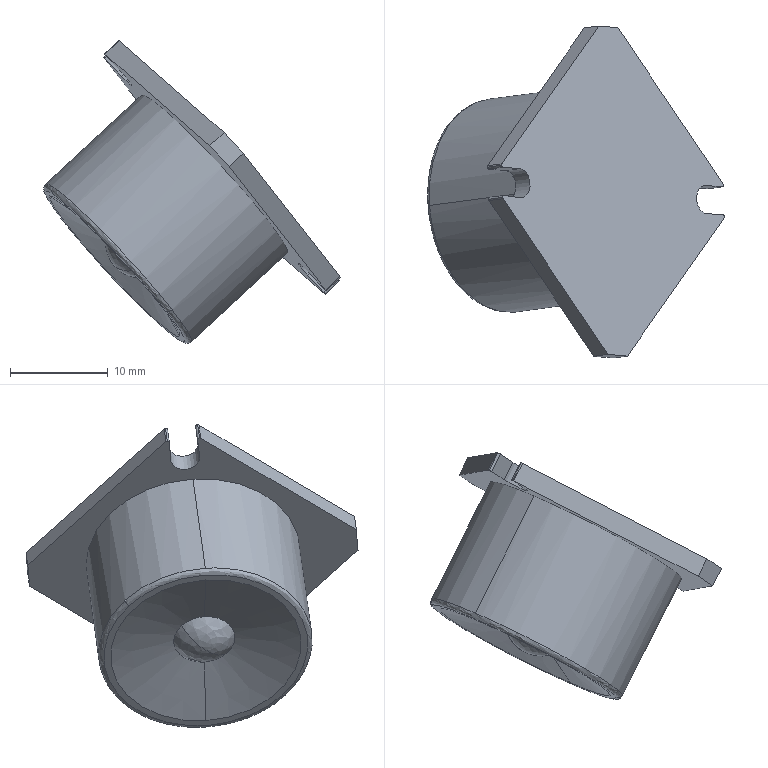Part | SolidWorks | features BaseBody 1 | 1 solid | 30 faces | box 30.403 x 34.026 x 31.023 mm | volume 6393 mm3 | plane 13 | cylinder 11 | spline 4 | cone 2 | commonest cylinder face diameters 0.4 x6 2.893 x2 22 x2 3.001 x1
STEP:
#1=CARTESIAN_POINT('',(690.687,-190.976,213.817));
#2=VERTEX_POINT('',#1);
#3=CARTESIAN_POINT('',(690.722,-190.926,213.773));
#4=VERTEX_POINT('',#3);
#5=CARTESIAN_POINT('',(690.687,-190.976,213.817));
#6=CARTESIAN_POINT('',(690.699,-190.959,213.802));
#7=CARTESIAN_POINT('',(690.71,-190.943,213.787));
#8=CARTESIAN_POINT('',(690.722,-190.926,213.773));
#9=(BOUNDED_CURVE()B_SPLINE_CURVE(3,(#5,#6,#7,#8),.UNSPECIFIED.,.F.,.F.)B_SPLINE_CURVE_WITH_KNOTS((4,4),(0.,0.002168),.UNSPECIFIED.)CURVE()GEOMETRIC_REPRESENTATION_ITEM()RATIONAL_B_SPLINE_CURVE((1.,1.,1.,1.))REPRESENTATION_ITEM(''));
#10=EDGE_CURVE('',#2,#4,#9,.T.);
#11=ORIENTED_EDGE('',*,*,#10,.T.);
#12=CARTESIAN_POINT('',(690.606,-191.348,213.217));
#13=VERTEX_POINT('',#12);
#14=CARTESIAN_POINT('',(690.722,-190.926,213.773));
#15=CARTESIAN_POINT('',(690.682,-190.932,213.735));
#16=CARTESIAN_POINT('',(690.597,-190.96,213.637));
#17=CARTESIAN_POINT('',(690.522,-191.062,213.467));
#18=CARTESIAN_POINT('',(690.529,-191.207,213.313));
#19=CARTESIAN_POINT('',(690.579,-191.307,213.241));
#20=CARTESIAN_POINT('',(690.606,-191.348,213.217));
#21=B_SPLINE_CURVE_WITH_KNOTS('',3,(#14,#15,#16,#17,#18,#19,#20),.UNSPECIFIED.,.F.,.F.,(4,1,1,1,4),(0.06704,0.25,0.5,0.75,0.933),.UNSPECIFIED.);
#22=EDGE_CURVE('',#4,#13,#21,.T.);
#23=ORIENTED_EDGE('',*,*,#22,.T.);
#24=CARTESIAN_POINT('',(690.573,-191.395,213.259));
#25=VERTEX_POINT('',#24);
#26=CARTESIAN_POINT('',(690.573,-191.395,213.259));
#27=CARTESIAN_POINT('',(690.584,-191.38,213.245));
#28=CARTESIAN_POINT('',(690.595,-191.364,213.231));
#29=CARTESIAN_POINT('',(690.606,-191.348,213.217));
#30=B_SPLINE_CURVE_WITH_KNOTS('',3,(#26,#27,#28,#29),.UNSPECIFIED.,.F.,.F.,(4,4),(0.,1.),.UNSPECIFIED.);
#31=EDGE_CURVE('',#25,#13,#30,.T.);
#32=ORIENTED_EDGE('',*,*,#31,.F.);
#33=CARTESIAN_POINT('',(701.095,-207.085,204.088));
#34=VERTEX_POINT('',#33);
#35=CARTESIAN_POINT('',(701.095,-207.085,204.088));
#36=CARTESIAN_POINT('',(700.775,-207.536,204.497));
#37=CARTESIAN_POINT('',(700.424,-207.933,204.932));
#38=CARTESIAN_POINT('',(699.662,-208.616,205.85));
#39=CARTESIAN_POINT('',(699.257,-208.897,206.327));
#40=CARTESIAN_POINT('',(698.403,-209.337,207.311));
#41=CARTESIAN_POINT('',(697.961,-209.491,207.811));
#42=CARTESIAN_POINT('',(697.047,-209.67,208.823));
#43=CARTESIAN_POINT('',(696.583,-209.692,209.327));
#44=CARTESIAN_POINT('',(695.645,-209.603,210.328));
#45=CARTESIAN_POINT('',(695.178,-209.492,210.817));
#46=CARTESIAN_POINT('',(694.251,-209.139,211.77));
#47=CARTESIAN_POINT('',(693.798,-208.899,212.225));
#48=CARTESIAN_POINT('',(692.918,-208.295,213.092));
#49=CARTESIAN_POINT('',(692.497,-207.936,213.496));
#50=CARTESIAN_POINT('',(691.697,-207.104,214.244));
#51=CARTESIAN_POINT('',(691.324,-206.638,214.582));
#52=CARTESIAN_POINT('',(690.635,-205.611,215.182));
#53=CARTESIAN_POINT('',(690.325,-205.057,215.44));
#54=CARTESIAN_POINT('',(689.773,-203.873,215.871));
#55=CARTESIAN_POINT('',(689.536,-203.253,216.039));
#56=CARTESIAN_POINT('',(689.143,-201.958,216.283));
#57=CARTESIAN_POINT('',(688.99,-201.294,216.356));
#58=CARTESIAN_POINT('',(688.77,-199.937,216.403));
#59=CARTESIAN_POINT('',(688.706,-199.255,216.377));
#60=CARTESIAN_POINT('',(688.668,-197.889,216.227));
#61=CARTESIAN_POINT('',(688.695,-197.215,216.103));
#62=CARTESIAN_POINT('',(688.841,-195.891,215.761));
#63=CARTESIAN_POINT('',(688.958,-195.252,215.544));
#64=CARTESIAN_POINT('',(689.282,-194.021,215.022));
#65=CARTESIAN_POINT('',(689.485,-193.44,214.721));
#66=CARTESIAN_POINT('',(689.974,-192.35,214.041));
#67=CARTESIAN_POINT('',(690.255,-191.85,213.667));
#68=CARTESIAN_POINT('',(690.573,-191.395,213.259));
#69=B_SPLINE_CURVE_WITH_KNOTS('',3,(#35,#36,#37,#38,#39,#40,#41,#42,#43,#44,#45,#46,#47,#48,#49,#50,#51,#52,#53,#54,#55,#56,#57,#58,#59,#60,#61,#62,#63,#64,#65,#66,#67,#68),.UNSPECIFIED.,.F.,.F.,(4,2,2,2,2,2,2,2,2,2,2,2,2,2,2,2,4),(0.,0.0625,0.125,0.1875,0.25,0.3125,0.375,0.4375,0.5,0.5625,0.625,0.6875,0.75,0.8125,0.875,0.9375,1.),.UNSPECIFIED.);
#70=EDGE_CURVE('',#34,#25,#69,.T.);
#71=ORIENTED_EDGE('',*,*,#70,.F.);
#72=CARTESIAN_POINT('',(701.71,-207.413,204.209));
#73=VERTEX_POINT('',#72);
#74=CARTESIAN_POINT('',(701.71,-207.413,204.209));
#75=CARTESIAN_POINT('',(701.669,-207.418,204.171));
#76=CARTESIAN_POINT('',(701.563,-207.414,204.092));
#77=CARTESIAN_POINT('',(701.376,-207.347,204.02));
#78=CARTESIAN_POINT('',(701.204,-207.223,204.022));
#79=CARTESIAN_POINT('',(701.123,-207.127,204.064));
#80=CARTESIAN_POINT('',(701.095,-207.085,204.088));
#81=B_SPLINE_CURVE_WITH_KNOTS('',3,(#74,#75,#76,#77,#78,#79,#80),.UNSPECIFIED.,.F.,.F.,(4,1,1,1,4),(0.06704,0.25,0.5,0.75,0.933),.UNSPECIFIED.);
#82=EDGE_CURVE('',#73,#34,#81,.T.);
#83=ORIENTED_EDGE('',*,*,#82,.F.);
#84=CARTESIAN_POINT('',(688.744,-199.17,217.063));
#85=VERTEX_POINT('',#84);
#86=CARTESIAN_POINT('',(701.71,-207.413,204.209));
#87=CARTESIAN_POINT('',(696.604,-214.6,210.731));
#88=CARTESIAN_POINT('',(689.506,-210.087,217.768));
#89=CARTESIAN_POINT('',(688.744,-199.17,217.063));
#90=(BOUNDED_CURVE()B_SPLINE_CURVE(3,(#86,#87,#88,#89),.UNSPECIFIED.,.F.,.F.)B_SPLINE_CURVE_WITH_KNOTS((4,4),(0.002168,0.7309),.UNSPECIFIED.)CURVE()GEOMETRIC_REPRESENTATION_ITEM()RATIONAL_B_SPLINE_CURVE((1.,0.6089,0.6089,1.))REPRESENTATION_ITEM(''));
#91=EDGE_CURVE('',#73,#85,#90,.T.);
#92=ORIENTED_EDGE('',*,*,#91,.T.);
#93=CARTESIAN_POINT('',(688.744,-199.17,217.063));
#94=CARTESIAN_POINT('',(688.522,-195.988,216.858));
#95=CARTESIAN_POINT('',(689.21,-193.086,215.708));
#96=CARTESIAN_POINT('',(690.687,-190.976,213.817));
#97=(BOUNDED_CURVE()B_SPLINE_CURVE(3,(#93,#94,#95,#96),.UNSPECIFIED.,.F.,.F.)B_SPLINE_CURVE_WITH_KNOTS((4,4),(0.7309,1.),.UNSPECIFIED.)CURVE()GEOMETRIC_REPRESENTATION_ITEM()RATIONAL_B_SPLINE_CURVE((1.,0.9413,0.9413,1.))REPRESENTATION_ITEM(''));
#98=EDGE_CURVE('',#85,#2,#97,.T.);
#99=ORIENTED_EDGE('',*,*,#98,.T.);
#100=EDGE_LOOP('',(#11,#23,#32,#71,#83,#92,#99));
#101=FACE_OUTER_BOUND('',#100,.T.);
#102=CARTESIAN_POINT('',(701.71,-207.413,204.209));
#103=CARTESIAN_POINT('',(691.467,-221.83,217.293));
#104=CARTESIAN_POINT('',(680.479,-205.344,226.857));
#105=CARTESIAN_POINT('',(690.722,-190.926,213.772));
#106=CARTESIAN_POINT('',(701.669,-207.418,204.171));
#107=CARTESIAN_POINT('',(691.426,-221.835,217.256));
#108=CARTESIAN_POINT('',(680.438,-205.349,226.82));
#109=CARTESIAN_POINT('',(690.682,-190.932,213.735));
#110=CARTESIAN_POINT('',(701.563,-207.414,204.092));
#111=CARTESIAN_POINT('',(691.34,-221.803,217.151));
#112=CARTESIAN_POINT('',(680.374,-205.349,226.696));
#113=CARTESIAN_POINT('',(690.597,-190.96,213.637));
#114=CARTESIAN_POINT('',(701.376,-207.347,204.02));
#115=CARTESIAN_POINT('',(691.257,-221.589,216.945));
#116=CARTESIAN_POINT('',(680.403,-205.303,226.392));
#117=CARTESIAN_POINT('',(690.522,-191.062,213.467));
#118=CARTESIAN_POINT('',(701.204,-207.223,204.022));
#119=CARTESIAN_POINT('',(691.253,-221.229,216.733));
#120=CARTESIAN_POINT('',(680.578,-205.213,226.024));
#121=CARTESIAN_POINT('',(690.529,-191.207,213.313));
#122=CARTESIAN_POINT('',(701.123,-207.127,204.064));
#123=CARTESIAN_POINT('',(691.293,-220.962,216.62));
#124=CARTESIAN_POINT('',(680.75,-205.142,225.797));
#125=CARTESIAN_POINT('',(690.579,-191.307,213.241));
#126=CARTESIAN_POINT('',(701.095,-207.085,204.088));
#127=CARTESIAN_POINT('',(691.317,-220.848,216.578));
#128=CARTESIAN_POINT('',(680.829,-205.111,225.707));
#129=CARTESIAN_POINT('',(690.606,-191.348,213.217));
#130=(BOUNDED_SURFACE()B_SPLINE_SURFACE(3,3,((#102,#103,#104,#105),(#106,#107,#108,#109),(#110,#111,#112,#113),(#114,#115,#116,#117),(#118,#119,#120,#121),(#122,#123,#124,#125),(#126,#127,#128,#129)),.UNSPECIFIED.,.F.,.F.,.T.)B_SPLINE_SURFACE_WITH_KNOTS((4,1,1,1,4),(4,4),(0.06704,0.25,0.5,0.75,0.933),(0.,1.),.UNSPECIFIED.)GEOMETRIC_REPRESENTATION_ITEM()RATIONAL_B_SPLINE_SURFACE(((1.,0.3333,0.3333,1.),(1.,0.3333,0.3333,1.),(1.,0.3333,0.3333,1.),(1.,0.3333,0.3333,1.),(1.,0.3333,0.3333,1.),(1.,0.3333,0.3333,1.),(1.,0.3333,0.3333,1.)))REPRESENTATION_ITEM('')SURFACE());
#131=ADVANCED_FACE('',(#101),#130,.F.);
#132=CARTESIAN_POINT('',(698.658,-201.411,208.396));
#133=VERTEX_POINT('',#132);
#134=CARTESIAN_POINT('',(699.215,-199.059,207.464));
#135=VERTEX_POINT('',#134);
#136=CARTESIAN_POINT('',(697.07,-199.059,209.781));
#137=DIRECTION('',(0.7306,0.09465,0.6762));
#138=DIRECTION('',(-0.5026,0.7449,0.4388));
#139=AXIS2_PLACEMENT_3D('',#136,#137,#138);
#140=CIRCLE('',#139,3.158);
#141=EDGE_CURVE('',#133,#135,#140,.T.);
#142=ORIENTED_EDGE('',*,*,#141,.F.);
#143=CARTESIAN_POINT('',(695.851,-199.217,208.652));
#144=VERTEX_POINT('',#143);
#145=CARTESIAN_POINT('',(698.658,-201.411,208.396));
#146=CARTESIAN_POINT('',(698.399,-201.312,208.305));
#147=CARTESIAN_POINT('',(697.861,-201.058,208.168));
#148=CARTESIAN_POINT('',(697.085,-200.545,208.134));
#149=CARTESIAN_POINT('',(696.385,-199.915,208.29));
#150=CARTESIAN_POINT('',(696.009,-199.452,208.514));
#151=CARTESIAN_POINT('',(695.851,-199.217,208.652));
#152=B_SPLINE_CURVE_WITH_KNOTS('',3,(#145,#146,#147,#148,#149,#150,#151),.UNSPECIFIED.,.F.,.F.,(4,1,1,1,4),(0.01961,0.25,0.5,0.75,1.),.UNSPECIFIED.);
#153=EDGE_CURVE('',#133,#144,#152,.T.);
#154=ORIENTED_EDGE('',*,*,#153,.T.);
#155=CARTESIAN_POINT('',(695.483,-196.707,211.167));
#156=VERTEX_POINT('',#155);
#157=CARTESIAN_POINT('',(695.483,-196.707,211.167));
#158=CARTESIAN_POINT('',(695.39,-196.851,210.932));
#159=CARTESIAN_POINT('',(695.253,-197.193,210.444));
#160=CARTESIAN_POINT('',(695.238,-197.808,209.747));
#161=CARTESIAN_POINT('',(695.432,-198.503,209.122));
#162=CARTESIAN_POINT('',(695.692,-198.982,208.791));
#163=CARTESIAN_POINT('',(695.851,-199.217,208.652));
#164=B_SPLINE_CURVE_WITH_KNOTS('',3,(#157,#158,#159,#160,#161,#162,#163),.UNSPECIFIED.,.F.,.F.,(4,1,1,1,4),(0.01961,0.25,0.5,0.75,1.),.UNSPECIFIED.);
#165=EDGE_CURVE('',#156,#144,#164,.T.);
#166=ORIENTED_EDGE('',*,*,#165,.F.);
#167=CARTESIAN_POINT('',(697.07,-199.059,209.781));
#168=DIRECTION('',(0.7306,0.09465,0.6762));
#169=DIRECTION('',(-0.5026,0.7449,0.4388));
#170=AXIS2_PLACEMENT_3D('',#167,#168,#169);
#171=CIRCLE('',#170,3.158);
#172=EDGE_CURVE('',#135,#156,#171,.T.);
#173=ORIENTED_EDGE('',*,*,#172,.F.);
#174=EDGE_LOOP('',(#142,#154,#166,#173));
#175=FACE_OUTER_BOUND('',#174,.T.);
#176=CARTESIAN_POINT('',(695.483,-196.707,211.167));
#177=CARTESIAN_POINT('',(698.402,-192.536,207.43));
#178=CARTESIAN_POINT('',(701.577,-197.24,204.658));
#179=CARTESIAN_POINT('',(698.658,-201.411,208.396));
#180=CARTESIAN_POINT('',(695.39,-196.851,210.932));
#181=CARTESIAN_POINT('',(698.157,-192.897,207.389));
#182=CARTESIAN_POINT('',(701.167,-197.357,204.762));
#183=CARTESIAN_POINT('',(698.399,-201.312,208.305));
#184=CARTESIAN_POINT('',(695.253,-197.193,210.444));
#185=CARTESIAN_POINT('',(697.651,-193.766,207.374));
#186=CARTESIAN_POINT('',(700.259,-197.631,205.097));
#187=CARTESIAN_POINT('',(697.861,-201.058,208.168));
#188=CARTESIAN_POINT('',(695.238,-197.808,209.747));
#189=CARTESIAN_POINT('',(696.937,-195.381,207.572));
#190=CARTESIAN_POINT('',(698.784,-198.118,205.959));
#191=CARTESIAN_POINT('',(697.085,-200.545,208.134));
#192=CARTESIAN_POINT('',(695.432,-198.503,209.122));
#193=CARTESIAN_POINT('',(696.308,-197.252,208.));
#194=CARTESIAN_POINT('',(697.261,-198.664,207.168));
#195=CARTESIAN_POINT('',(696.385,-199.915,208.29));
#196=CARTESIAN_POINT('',(695.692,-198.982,208.791));
#197=CARTESIAN_POINT('',(695.984,-198.564,208.417));
#198=CARTESIAN_POINT('',(696.301,-199.035,208.14));
#199=CARTESIAN_POINT('',(696.009,-199.452,208.514));
#200=CARTESIAN_POINT('',(695.851,-199.217,208.652));
#201=CARTESIAN_POINT('',(695.851,-199.217,208.652));
#202=CARTESIAN_POINT('',(695.851,-199.217,208.652));
#203=CARTESIAN_POINT('',(695.851,-199.217,208.652));
#204=(BOUNDED_SURFACE()B_SPLINE_SURFACE(3,3,((#176,#177,#178,#179),(#180,#181,#182,#183),(#184,#185,#186,#187),(#188,#189,#190,#191),(#192,#193,#194,#195),(#196,#197,#198,#199),(#200,#201,#202,#203)),.UNSPECIFIED.,.F.,.F.,.T.)B_SPLINE_SURFACE_WITH_KNOTS((4,1,1,1,4),(4,4),(0.01961,0.25,0.5,0.75,1.),(0.,1.),.UNSPECIFIED.)GEOMETRIC_REPRESENTATION_ITEM()RATIONAL_B_SPLINE_SURFACE(((1.,0.3333,0.3333,1.),(1.,0.3333,0.3333,1.),(1.,0.3333,0.3333,1.),(1.,0.3333,0.3333,1.),(1.,0.3333,0.3333,1.),(1.,0.3333,0.3333,1.),(1.,0.3333,0.3333,1.)))REPRESENTATION_ITEM('')SURFACE());
#205=ADVANCED_FACE('',(#175),#204,.F.);
#206=CARTESIAN_POINT('',(717.052,-197.111,209.113));
#207=VERTEX_POINT('',#206);
#208=CARTESIAN_POINT('',(716.114,-198.548,210.327));
#209=VERTEX_POINT('',#208);
#210=CARTESIAN_POINT('',(717.096,-198.548,209.266));
#211=DIRECTION('',(0.7306,0.09465,0.6762));
#212=DIRECTION('',(-0.6793,0.,0.7339));
#213=AXIS2_PLACEMENT_3D('',#210,#211,#212);
#214=CIRCLE('',#213,1.446);
#215=EDGE_CURVE('',#207,#209,#214,.T.);
#216=ORIENTED_EDGE('',*,*,#215,.T.);
#217=CARTESIAN_POINT('',(714.653,-198.738,208.975));
#218=VERTEX_POINT('',#217);
#219=CARTESIAN_POINT('',(716.114,-198.548,210.327));
#220=DIRECTION('',(-0.7306,-0.09465,-0.6762));
#221=VECTOR('',#220,1000.);
#222=LINE('',#219,#221);
#223=EDGE_CURVE('',#209,#218,#222,.T.);
#224=ORIENTED_EDGE('',*,*,#223,.T.);
#225=CARTESIAN_POINT('',(715.591,-197.3,207.76));
#226=VERTEX_POINT('',#225);
#227=CARTESIAN_POINT('',(715.635,-198.738,207.913));
#228=DIRECTION('',(-0.7306,-0.09465,-0.6762));
#229=DIRECTION('',(-0.6793,0.,0.7339));
#230=AXIS2_PLACEMENT_3D('',#227,#228,#229);
#231=CIRCLE('',#230,1.446);
#232=EDGE_CURVE('',#218,#226,#231,.T.);
#233=ORIENTED_EDGE('',*,*,#232,.T.);
#234=CARTESIAN_POINT('',(716.321,-197.205,208.437));
#235=DIRECTION('',(0.7306,0.09465,0.6762));
#236=VECTOR('',#235,1000.);
#237=LINE('',#234,#236);
#238=EDGE_CURVE('',#226,#207,#237,.T.);
#239=ORIENTED_EDGE('',*,*,#238,.T.);
#240=EDGE_LOOP('',(#216,#224,#233,#239));
#241=FACE_OUTER_BOUND('',#240,.T.);
#242=CARTESIAN_POINT('',(717.096,-198.548,209.266));
#243=DIRECTION('',(-0.7306,-0.09465,-0.6762));
#244=DIRECTION('',(-0.6793,0.,0.7339));
#245=AXIS2_PLACEMENT_3D('',#242,#243,#244);
#246=CYLINDRICAL_SURFACE('',#245,1.446);
#247=ADVANCED_FACE('',(#241),#246,.F.);
#248=CARTESIAN_POINT('',(696.132,-195.082,231.431));
#249=VERTEX_POINT('',#248);
#250=CARTESIAN_POINT('',(696.274,-195.281,231.305));
#251=VERTEX_POINT('',#250);
#252=CARTESIAN_POINT('',(696.268,-195.082,231.284));
#253=DIRECTION('',(0.7306,0.09465,0.6762));
#254=DIRECTION('',(-0.6793,0.,0.7339));
#255=AXIS2_PLACEMENT_3D('',#252,#253,#254);
#256=CIRCLE('',#255,0.2);
#257=EDGE_CURVE('',#249,#251,#256,.T.);
#258=ORIENTED_EDGE('',*,*,#257,.F.);
#259=CARTESIAN_POINT('',(694.671,-195.272,230.078));
#260=VERTEX_POINT('',#259);
#261=CARTESIAN_POINT('',(696.132,-195.082,231.431));
#262=DIRECTION('',(-0.7306,-0.09465,-0.6762));
#263=VECTOR('',#262,1000.);
#264=LINE('',#261,#263);
#265=EDGE_CURVE('',#249,#260,#264,.T.);
#266=ORIENTED_EDGE('',*,*,#265,.T.);
#267=CARTESIAN_POINT('',(694.813,-195.47,229.953));
#268=VERTEX_POINT('',#267);
#269=CARTESIAN_POINT('',(694.807,-195.272,229.931));
#270=DIRECTION('',(-0.7306,-0.09465,-0.6762));
#271=DIRECTION('',(-0.6793,0.,0.7339));
#272=AXIS2_PLACEMENT_3D('',#269,#270,#271);
#273=CIRCLE('',#272,0.2);
#274=EDGE_CURVE('',#268,#260,#273,.T.);
#275=ORIENTED_EDGE('',*,*,#274,.F.);
#276=CARTESIAN_POINT('',(695.543,-195.376,230.629));
#277=DIRECTION('',(0.7306,0.09465,0.6762));
#278=VECTOR('',#277,1000.);
#279=LINE('',#276,#278);
#280=EDGE_CURVE('',#268,#251,#279,.T.);
#281=ORIENTED_EDGE('',*,*,#280,.T.);
#282=EDGE_LOOP('',(#258,#266,#275,#281));
#283=FACE_OUTER_BOUND('',#282,.T.);
#284=CARTESIAN_POINT('',(696.268,-195.082,231.284));
#285=DIRECTION('',(-0.7306,-0.09465,-0.6762));
#286=DIRECTION('',(-0.6793,0.,0.7339));
#287=AXIS2_PLACEMENT_3D('',#284,#285,#286);
#288=CYLINDRICAL_SURFACE('',#287,0.2);
#289=ADVANCED_FACE('',(#283),#288,.T.);
#290=CARTESIAN_POINT('',(696.237,-198.374,231.778));
#291=VERTEX_POINT('',#290);
#292=CARTESIAN_POINT('',(696.28,-198.506,231.749));
#293=VERTEX_POINT('',#292);
#294=CARTESIAN_POINT('',(696.373,-198.374,231.631));
#295=DIRECTION('',(0.7306,0.09465,0.6762));
#296=DIRECTION('',(-0.6793,0.,0.7339));
#297=AXIS2_PLACEMENT_3D('',#294,#295,#296);
#298=CIRCLE('',#297,0.2);
#299=EDGE_CURVE('',#291,#293,#298,.T.);
#300=ORIENTED_EDGE('',*,*,#299,.F.);
#301=CARTESIAN_POINT('',(694.776,-198.563,230.425));
#302=VERTEX_POINT('',#301);
#303=CARTESIAN_POINT('',(696.237,-198.374,231.778));
#304=DIRECTION('',(-0.7306,-0.09465,-0.6762));
#305=VECTOR('',#304,1000.);
#306=LINE('',#303,#305);
#307=EDGE_CURVE('',#291,#302,#306,.T.);
#308=ORIENTED_EDGE('',*,*,#307,.T.);
#309=CARTESIAN_POINT('',(694.819,-198.695,230.397));
#310=VERTEX_POINT('',#309);
#311=CARTESIAN_POINT('',(694.912,-198.563,230.279));
#312=DIRECTION('',(-0.7306,-0.09465,-0.6762));
#313=DIRECTION('',(-0.6793,0.,0.7339));
#314=AXIS2_PLACEMENT_3D('',#311,#312,#313);
#315=CIRCLE('',#314,0.2);
#316=EDGE_CURVE('',#310,#302,#315,.T.);
#317=ORIENTED_EDGE('',*,*,#316,.F.);
#318=CARTESIAN_POINT('',(695.55,-198.6,231.073));
#319=DIRECTION('',(0.7306,0.09465,0.6762));
#320=VECTOR('',#319,1000.);
#321=LINE('',#318,#320);
#322=EDGE_CURVE('',#310,#293,#321,.T.);
#323=ORIENTED_EDGE('',*,*,#322,.T.);
#324=EDGE_LOOP('',(#300,#308,#317,#323));
#325=FACE_OUTER_BOUND('',#324,.T.);
#326=CARTESIAN_POINT('',(696.373,-198.374,231.631));
#327=DIRECTION('',(-0.7306,-0.09465,-0.6762));
#328=DIRECTION('',(-0.6793,0.,0.7339));
#329=AXIS2_PLACEMENT_3D('',#326,#327,#328);
#330=CYLINDRICAL_SURFACE('',#329,0.2);
#331=ADVANCED_FACE('',(#325),#330,.T.);
#332=CARTESIAN_POINT('',(713.551,-197.892,210.047));
#333=VERTEX_POINT('',#332);
#334=CARTESIAN_POINT('',(698.607,-197.892,226.192));
#335=VERTEX_POINT('',#334);
#336=CARTESIAN_POINT('',(706.079,-197.892,218.12));
#337=DIRECTION('',(0.7306,0.09465,0.6762));
#338=DIRECTION('',(-0.6793,0.,0.7339));
#339=AXIS2_PLACEMENT_3D('',#336,#337,#338);
#340=CIRCLE('',#339,11.);
#341=EDGE_CURVE('',#333,#335,#340,.T.);
#342=ORIENTED_EDGE('',*,*,#341,.F.);
#343=CARTESIAN_POINT('',(703.688,-199.17,200.918));
#344=VERTEX_POINT('',#343);
#345=CARTESIAN_POINT('',(713.551,-197.892,210.047));
#346=DIRECTION('',(-0.7306,-0.09465,-0.6762));
#347=VECTOR('',#346,1000.);
#348=LINE('',#345,#347);
#349=EDGE_CURVE('',#333,#344,#348,.T.);
#350=ORIENTED_EDGE('',*,*,#349,.T.);
#351=CARTESIAN_POINT('',(690.722,-190.926,213.773));
#352=CARTESIAN_POINT('',(695.828,-183.739,207.25));
#353=CARTESIAN_POINT('',(702.926,-188.252,200.213));
#354=CARTESIAN_POINT('',(703.688,-199.17,200.918));
#355=(BOUNDED_CURVE()B_SPLINE_CURVE(3,(#351,#352,#353,#354),.UNSPECIFIED.,.F.,.F.)B_SPLINE_CURVE_WITH_KNOTS((4,4),(0.002168,0.7309),.UNSPECIFIED.)CURVE()GEOMETRIC_REPRESENTATION_ITEM()RATIONAL_B_SPLINE_CURVE((1.,0.6089,0.6089,1.))REPRESENTATION_ITEM(''));
#356=EDGE_CURVE('',#4,#344,#355,.T.);
#357=ORIENTED_EDGE('',*,*,#356,.F.);
#358=ORIENTED_EDGE('',*,*,#10,.F.);
#359=ORIENTED_EDGE('',*,*,#98,.F.);
#360=CARTESIAN_POINT('',(698.607,-197.892,226.192));
#361=DIRECTION('',(-0.7306,-0.09465,-0.6762));
#362=VECTOR('',#361,1000.);
#363=LINE('',#360,#362);
#364=EDGE_CURVE('',#335,#85,#363,.T.);
#365=ORIENTED_EDGE('',*,*,#364,.F.);
#366=EDGE_LOOP('',(#342,#350,#357,#358,#359,#365));
#367=FACE_OUTER_BOUND('',#366,.T.);
#368=CARTESIAN_POINT('',(706.079,-197.892,218.12));
#369=DIRECTION('',(-0.7306,-0.09465,-0.6762));
#370=DIRECTION('',(-0.6793,0.,0.7339));
#371=AXIS2_PLACEMENT_3D('',#368,#369,#370);
#372=CYLINDRICAL_SURFACE('',#371,11.);
#373=ADVANCED_FACE('',(#367),#372,.T.);
#374=CARTESIAN_POINT('',(694.925,-199.059,212.099));
#375=VERTEX_POINT('',#374);
#376=CARTESIAN_POINT('',(697.07,-199.059,209.781));
#377=DIRECTION('',(0.7306,0.09465,0.6762));
#378=DIRECTION('',(-0.5026,0.7449,0.4388));
#379=AXIS2_PLACEMENT_3D('',#376,#377,#378);
#380=CIRCLE('',#379,3.158);
#381=EDGE_CURVE('',#375,#133,#380,.T.);
#382=ORIENTED_EDGE('',*,*,#381,.T.);
#383=ORIENTED_EDGE('',*,*,#141,.T.);
#384=CARTESIAN_POINT('',(702.52,-199.217,201.447));
#385=VERTEX_POINT('',#384);
#386=CARTESIAN_POINT('',(699.215,-199.059,207.464));
#387=DIRECTION('',(0.4812,-0.02301,-0.8763));
#388=VECTOR('',#387,1000.);
#389=LINE('',#386,#388);
#390=EDGE_CURVE('',#135,#385,#389,.T.);
#391=ORIENTED_EDGE('',*,*,#390,.T.);
#392=CARTESIAN_POINT('',(689.181,-199.217,215.858));
#393=VERTEX_POINT('',#392);
#394=CARTESIAN_POINT('',(695.851,-199.217,208.652));
#395=DIRECTION('',(0.7306,0.09465,0.6762));
#396=DIRECTION('',(-0.6793,0.,0.7339));
#397=AXIS2_PLACEMENT_3D('',#394,#395,#396);
#398=CIRCLE('',#397,9.818);
#399=EDGE_CURVE('',#393,#385,#398,.T.);
#400=ORIENTED_EDGE('',*,*,#399,.F.);
#401=CARTESIAN_POINT('',(694.925,-199.059,212.099));
#402=DIRECTION('',(-0.8365,-0.02301,0.5474));
#403=VECTOR('',#402,1000.);
#404=LINE('',#401,#403);
#405=EDGE_CURVE('',#375,#393,#404,.T.);
#406=ORIENTED_EDGE('',*,*,#405,.F.);
#407=EDGE_LOOP('',(#382,#383,#391,#400,#406));
#408=FACE_OUTER_BOUND('',#407,.T.);
#409=CARTESIAN_POINT('',(697.07,-199.059,209.781));
#410=DIRECTION('',(-0.7306,-0.09465,-0.6762));
#411=DIRECTION('',(-0.6793,0.,0.7339));
#412=AXIS2_PLACEMENT_3D('',#409,#410,#411);
#413=CONICAL_SURFACE('',#412,3.158,1.325);
#414=ADVANCED_FACE('',(#408),#413,.F.);
#415=CARTESIAN_POINT('',(697.969,-195.422,229.493));
#416=VERTEX_POINT('',#415);
#417=CARTESIAN_POINT('',(696.232,-195.278,231.349));
#418=DIRECTION('',(-0.6821,0.05658,0.729));
#419=VECTOR('',#418,1000.);
#420=LINE('',#417,#419);
#421=EDGE_CURVE('',#416,#251,#420,.T.);
#422=ORIENTED_EDGE('',*,*,#421,.F.);
#423=CARTESIAN_POINT('',(698.024,-198.4,229.851));
#424=VERTEX_POINT('',#423);
#425=CARTESIAN_POINT('',(698.016,-196.913,229.652));
#426=DIRECTION('',(0.7306,0.09465,0.6762));
#427=DIRECTION('',(-0.6793,0.,0.7339));
#428=AXIS2_PLACEMENT_3D('',#425,#426,#427);
#429=CIRCLE('',#428,1.501);
#430=EDGE_CURVE('',#424,#416,#429,.T.);
#431=ORIENTED_EDGE('',*,*,#430,.F.);
#432=CARTESIAN_POINT('',(696.372,-198.175,231.604));
#433=VERTEX_POINT('',#432);
#434=CARTESIAN_POINT('',(698.066,-198.406,229.807));
#435=DIRECTION('',(0.6828,-0.09294,-0.7247));
#436=VECTOR('',#435,1000.);
#437=LINE('',#434,#436);
#438=EDGE_CURVE('',#433,#424,#437,.T.);
#439=ORIENTED_EDGE('',*,*,#438,.F.);
#440=CARTESIAN_POINT('',(696.373,-198.374,231.631));
#441=DIRECTION('',(0.7306,0.09465,0.6762));
#442=DIRECTION('',(-0.6793,0.,0.7339));
#443=AXIS2_PLACEMENT_3D('',#440,#441,#442);
#444=CIRCLE('',#443,0.2);
#445=EDGE_CURVE('',#433,#291,#444,.T.);
#446=ORIENTED_EDGE('',*,*,#445,.T.);
#447=ORIENTED_EDGE('',*,*,#299,.T.);
#448=CARTESIAN_POINT('',(707.038,-214.448,222.359));
#449=VERTEX_POINT('',#448);
#450=CARTESIAN_POINT('',(701.532,-206.288,227.165));
#451=DIRECTION('',(-0.5026,0.7449,0.4388));
#452=VECTOR('',#451,1000.);
#453=LINE('',#450,#452);
#454=EDGE_CURVE('',#449,#293,#453,.T.);
#455=ORIENTED_EDGE('',*,*,#454,.F.);
#456=CARTESIAN_POINT('',(709.011,-214.621,220.251));
#457=VERTEX_POINT('',#456);
#458=CARTESIAN_POINT('',(706.996,-214.444,222.403));
#459=DIRECTION('',(-0.6822,0.05972,0.7287));
#460=VECTOR('',#459,1000.);
#461=LINE('',#458,#460);
#462=EDGE_CURVE('',#457,#449,#461,.T.);
#463=ORIENTED_EDGE('',*,*,#462,.F.);
#464=CARTESIAN_POINT('',(718.913,-200.472,207.572));
#465=VERTEX_POINT('',#464);
#466=CARTESIAN_POINT('',(714.074,-207.386,213.768));
#467=DIRECTION('',(-0.4622,-0.6604,0.5918));
#468=VECTOR('',#467,1000.);
#469=LINE('',#466,#468);
#470=EDGE_CURVE('',#465,#457,#469,.T.);
#471=ORIENTED_EDGE('',*,*,#470,.F.);
#472=CARTESIAN_POINT('',(718.806,-200.124,207.639));
#473=VERTEX_POINT('',#472);
#474=CARTESIAN_POINT('',(718.812,-200.323,207.66));
#475=DIRECTION('',(0.7306,0.09465,0.6762));
#476=DIRECTION('',(-0.6793,0.,0.7339));
#477=AXIS2_PLACEMENT_3D('',#474,#475,#476);
#478=CIRCLE('',#477,0.2);
#479=EDGE_CURVE('',#465,#473,#478,.T.);
#480=ORIENTED_EDGE('',*,*,#479,.T.);
#481=CARTESIAN_POINT('',(717.141,-199.986,209.419));
#482=VERTEX_POINT('',#481);
#483=CARTESIAN_POINT('',(718.848,-200.127,207.595));
#484=DIRECTION('',(0.6821,-0.05658,-0.729));
#485=VECTOR('',#484,1000.);
#486=LINE('',#483,#485);
#487=EDGE_CURVE('',#482,#473,#486,.T.);
#488=ORIENTED_EDGE('',*,*,#487,.F.);
#489=CARTESIAN_POINT('',(717.096,-198.548,209.266));
#490=DIRECTION('',(0.7306,0.09465,0.6762));
#491=DIRECTION('',(-0.6793,0.,0.7339));
#492=AXIS2_PLACEMENT_3D('',#489,#490,#491);
#493=CIRCLE('',#492,1.446);
#494=EDGE_CURVE('',#209,#482,#493,.T.);
#495=ORIENTED_EDGE('',*,*,#494,.F.);
#496=ORIENTED_EDGE('',*,*,#215,.F.);
#497=CARTESIAN_POINT('',(718.726,-197.25,207.323));
#498=VERTEX_POINT('',#497);
#499=CARTESIAN_POINT('',(717.01,-197.107,209.157));
#500=DIRECTION('',(-0.6821,0.05658,0.729));
#501=VECTOR('',#500,1000.);
#502=LINE('',#499,#501);
#503=EDGE_CURVE('',#498,#207,#502,.T.);
#504=ORIENTED_EDGE('',*,*,#503,.F.);
#505=CARTESIAN_POINT('',(718.813,-196.919,207.183));
#506=VERTEX_POINT('',#505);
#507=CARTESIAN_POINT('',(718.72,-197.051,207.302));
#508=DIRECTION('',(0.7306,0.09465,0.6762));
#509=DIRECTION('',(-0.6793,0.,0.7339));
#510=AXIS2_PLACEMENT_3D('',#507,#508,#509);
#511=CIRCLE('',#510,0.2);
#512=EDGE_CURVE('',#498,#506,#511,.T.);
#513=ORIENTED_EDGE('',*,*,#512,.T.);
#514=CARTESIAN_POINT('',(708.043,-180.957,216.585));
#515=VERTEX_POINT('',#514);
#516=CARTESIAN_POINT('',(713.549,-189.117,211.779));
#517=DIRECTION('',(0.5026,-0.7449,-0.4388));
#518=VECTOR('',#517,1000.);
#519=LINE('',#516,#518);
#520=EDGE_CURVE('',#515,#506,#519,.T.);
#521=ORIENTED_EDGE('',*,*,#520,.F.);
#522=CARTESIAN_POINT('',(706.069,-180.784,218.693));
#523=VERTEX_POINT('',#522);
#524=CARTESIAN_POINT('',(708.084,-180.961,216.541));
#525=DIRECTION('',(0.6822,-0.05972,-0.7287));
#526=VECTOR('',#525,1000.);
#527=LINE('',#524,#526);
#528=EDGE_CURVE('',#523,#515,#527,.T.);
#529=ORIENTED_EDGE('',*,*,#528,.F.);
#530=CARTESIAN_POINT('',(696.167,-194.933,231.372));
#531=VERTEX_POINT('',#530);
#532=CARTESIAN_POINT('',(701.006,-188.019,225.176));
#533=DIRECTION('',(0.4622,0.6604,-0.5918));
#534=VECTOR('',#533,1000.);
#535=LINE('',#532,#534);
#536=EDGE_CURVE('',#531,#523,#535,.T.);
#537=ORIENTED_EDGE('',*,*,#536,.F.);
#538=CARTESIAN_POINT('',(696.268,-195.082,231.284));
#539=DIRECTION('',(0.7306,0.09465,0.6762));
#540=DIRECTION('',(-0.6793,0.,0.7339));
#541=AXIS2_PLACEMENT_3D('',#538,#539,#540);
#542=CIRCLE('',#541,0.2);
#543=EDGE_CURVE('',#531,#249,#542,.T.);
#544=ORIENTED_EDGE('',*,*,#543,.T.);
#545=ORIENTED_EDGE('',*,*,#257,.T.);
#546=EDGE_LOOP('',(#422,#431,#439,#446,#447,#455,#463,#471,#480,#488,#495,#496,#504,#513,#521,#529,#537,#544,#545));
#547=FACE_OUTER_BOUND('',#546,.T.);
#548=CARTESIAN_POINT('',(708.087,-216.703,221.541));
#549=DIRECTION('',(-0.7306,-0.09465,-0.6762));
#550=DIRECTION('',(-0.5026,0.7449,0.4388));
#551=AXIS2_PLACEMENT_3D('',#548,#549,#550);
#552=PLANE('',#551);
#553=ADVANCED_FACE('',(#547),#552,.F.);
#554=CARTESIAN_POINT('',(696.508,-195.611,228.141));
#555=VERTEX_POINT('',#554);
#556=CARTESIAN_POINT('',(695.66,-195.541,229.047));
#557=DIRECTION('',(-0.6821,0.05658,0.729));
#558=VECTOR('',#557,1000.);
#559=LINE('',#556,#558);
#560=EDGE_CURVE('',#555,#268,#559,.T.);
#561=ORIENTED_EDGE('',*,*,#560,.F.);
#562=CARTESIAN_POINT('',(697.239,-195.516,228.817));
#563=DIRECTION('',(-0.7306,-0.09465,-0.6762));
#564=VECTOR('',#563,1000.);
#565=LINE('',#562,#564);
#566=EDGE_CURVE('',#416,#555,#565,.T.);
#567=ORIENTED_EDGE('',*,*,#566,.F.);
#568=ORIENTED_EDGE('',*,*,#421,.T.);
#569=ORIENTED_EDGE('',*,*,#280,.F.);
#570=EDGE_LOOP('',(#561,#567,#568,#569));
#571=FACE_OUTER_BOUND('',#570,.T.);
#572=CARTESIAN_POINT('',(696.277,-195.272,231.39));
#573=DIRECTION('',(-0.03074,0.9939,-0.1059));
#574=DIRECTION('',(0.6821,-0.05658,-0.729));
#575=AXIS2_PLACEMENT_3D('',#572,#573,#574);
#576=PLANE('',#575);
#577=ADVANCED_FACE('',(#571),#576,.F.);
#578=ORIENTED_EDGE('',*,*,#566,.T.);
#579=CARTESIAN_POINT('',(696.563,-198.59,228.498));
#580=VERTEX_POINT('',#579);
#581=CARTESIAN_POINT('',(696.554,-197.102,228.299));
#582=DIRECTION('',(-0.7306,-0.09465,-0.6762));
#583=DIRECTION('',(-0.6793,0.,0.7339));
#584=AXIS2_PLACEMENT_3D('',#581,#582,#583);
#585=CIRCLE('',#584,1.501);
#586=EDGE_CURVE('',#555,#580,#585,.T.);
#587=ORIENTED_EDGE('',*,*,#586,.T.);
#588=CARTESIAN_POINT('',(697.294,-198.495,229.175));
#589=DIRECTION('',(0.7306,0.09465,0.6762));
#590=VECTOR('',#589,1000.);
#591=LINE('',#588,#590);
#592=EDGE_CURVE('',#580,#424,#591,.T.);
#593=ORIENTED_EDGE('',*,*,#592,.T.);
#594=ORIENTED_EDGE('',*,*,#430,.T.);
#595=EDGE_LOOP('',(#578,#587,#593,#594));
#596=FACE_OUTER_BOUND('',#595,.T.);
#597=CARTESIAN_POINT('',(698.016,-196.913,229.652));
#598=DIRECTION('',(-0.7306,-0.09465,-0.6762));
#599=DIRECTION('',(-0.6793,0.,0.7339));
#600=AXIS2_PLACEMENT_3D('',#597,#598,#599);
#601=CYLINDRICAL_SURFACE('',#600,1.501);
#602=ADVANCED_FACE('',(#596),#601,.F.);
#603=ORIENTED_EDGE('',*,*,#438,.T.);
#604=ORIENTED_EDGE('',*,*,#592,.F.);
#605=CARTESIAN_POINT('',(694.911,-198.365,230.252));
#606=VERTEX_POINT('',#605);
#607=CARTESIAN_POINT('',(695.737,-198.477,229.375));
#608=DIRECTION('',(0.6828,-0.09294,-0.7247));
#609=VECTOR('',#608,1000.);
#610=LINE('',#607,#609);
#611=EDGE_CURVE('',#606,#580,#610,.T.);
#612=ORIENTED_EDGE('',*,*,#611,.F.);
#613=CARTESIAN_POINT('',(695.641,-198.27,230.928));
#614=DIRECTION('',(-0.7306,-0.09465,-0.6762));
#615=VECTOR('',#614,1000.);
#616=LINE('',#613,#615);
#617=EDGE_CURVE('',#433,#606,#616,.T.);
#618=ORIENTED_EDGE('',*,*,#617,.F.);
#619=EDGE_LOOP('',(#603,#604,#612,#618));
#620=FACE_OUTER_BOUND('',#619,.T.);
#621=CARTESIAN_POINT('',(698.11,-198.4,229.848));
#622=DIRECTION('',(0.005744,-0.9912,0.1325));
#623=DIRECTION('',(-0.6828,0.09294,0.7247));
#624=AXIS2_PLACEMENT_3D('',#621,#622,#623);
#625=PLANE('',#624);
#626=ADVANCED_FACE('',(#620),#625,.F.);
#627=CARTESIAN_POINT('',(705.576,-214.637,221.006));
#628=VERTEX_POINT('',#627);
#629=CARTESIAN_POINT('',(700.198,-206.666,225.702));
#630=DIRECTION('',(-0.5026,0.7449,0.4388));
#631=VECTOR('',#630,1000.);
#632=LINE('',#629,#631);
#633=EDGE_CURVE('',#628,#310,#632,.T.);
#634=ORIENTED_EDGE('',*,*,#633,.F.);
#635=CARTESIAN_POINT('',(706.307,-214.543,221.683));
#636=DIRECTION('',(-0.7306,-0.09465,-0.6762));
#637=VECTOR('',#636,1000.);
#638=LINE('',#635,#637);
#639=EDGE_CURVE('',#449,#628,#638,.T.);
#640=ORIENTED_EDGE('',*,*,#639,.F.);
#641=ORIENTED_EDGE('',*,*,#454,.T.);
#642=ORIENTED_EDGE('',*,*,#322,.F.);
#643=EDGE_LOOP('',(#634,#640,#641,#642));
#644=FACE_OUTER_BOUND('',#643,.T.);
#645=CARTESIAN_POINT('',(696.11,-198.181,231.978));
#646=DIRECTION('',(0.4622,0.6604,-0.5918));
#647=DIRECTION('',(0.5026,-0.7449,-0.4388));
#648=AXIS2_PLACEMENT_3D('',#645,#646,#647);
#649=PLANE('',#648);
#650=ADVANCED_FACE('',(#644),#649,.F.);
#651=CARTESIAN_POINT('',(707.55,-214.81,218.898));
#652=VERTEX_POINT('',#651);
#653=CARTESIAN_POINT('',(708.28,-214.715,219.575));
#654=DIRECTION('',(-0.7306,-0.09465,-0.6762));
#655=VECTOR('',#654,1000.);
#656=LINE('',#653,#655);
#657=EDGE_CURVE('',#457,#652,#656,.T.);
#658=ORIENTED_EDGE('',*,*,#657,.F.);
#659=ORIENTED_EDGE('',*,*,#462,.T.);
#660=ORIENTED_EDGE('',*,*,#639,.T.);
#661=CARTESIAN_POINT('',(706.563,-214.724,219.952));
#662=DIRECTION('',(-0.6822,0.05972,0.7287));
#663=VECTOR('',#662,1000.);
#664=LINE('',#661,#663);
#665=EDGE_CURVE('',#652,#628,#664,.T.);
#666=ORIENTED_EDGE('',*,*,#665,.F.);
#667=EDGE_LOOP('',(#658,#659,#660,#666));
#668=FACE_OUTER_BOUND('',#667,.T.);
#669=CARTESIAN_POINT('',(707.04,-214.439,222.444));
#670=DIRECTION('',(-0.02858,0.9937,-0.1082));
#671=DIRECTION('',(0.6822,-0.05972,-0.7287));
#672=AXIS2_PLACEMENT_3D('',#669,#670,#671);
#673=PLANE('',#672);
#674=ADVANCED_FACE('',(#668),#673,.F.);
#675=ORIENTED_EDGE('',*,*,#470,.T.);
#676=ORIENTED_EDGE('',*,*,#657,.T.);
#677=CARTESIAN_POINT('',(717.452,-200.661,206.22));
#678=VERTEX_POINT('',#677);
#679=CARTESIAN_POINT('',(712.501,-207.736,212.559));
#680=DIRECTION('',(-0.4622,-0.6604,0.5918));
#681=VECTOR('',#680,1000.);
#682=LINE('',#679,#681);
#683=EDGE_CURVE('',#678,#652,#682,.T.);
#684=ORIENTED_EDGE('',*,*,#683,.F.);
#685=CARTESIAN_POINT('',(718.182,-200.566,206.896));
#686=DIRECTION('',(-0.7306,-0.09465,-0.6762));
#687=VECTOR('',#686,1000.);
#688=LINE('',#685,#687);
#689=EDGE_CURVE('',#465,#678,#688,.T.);
#690=ORIENTED_EDGE('',*,*,#689,.F.);
#691=EDGE_LOOP('',(#675,#676,#684,#690));
#692=FACE_OUTER_BOUND('',#691,.T.);
#693=CARTESIAN_POINT('',(708.857,-214.898,220.546));
#694=DIRECTION('',(-0.5026,0.7449,0.4388));
#695=DIRECTION('',(0.4622,0.6604,-0.5918));
#696=AXIS2_PLACEMENT_3D('',#693,#694,#695);
#697=PLANE('',#696);
#698=ADVANCED_FACE('',(#692),#697,.F.);
#699=CARTESIAN_POINT('',(715.68,-200.175,208.067));
#700=VERTEX_POINT('',#699);
#701=CARTESIAN_POINT('',(717.345,-200.313,206.287));
#702=VERTEX_POINT('',#701);
#703=CARTESIAN_POINT('',(716.512,-200.244,207.177));
#704=DIRECTION('',(0.6821,-0.05658,-0.729));
#705=VECTOR('',#704,1000.);
#706=LINE('',#703,#705);
#707=EDGE_CURVE('',#700,#702,#706,.T.);
#708=ORIENTED_EDGE('',*,*,#707,.F.);
#709=CARTESIAN_POINT('',(716.41,-200.081,208.743));
#710=DIRECTION('',(-0.7306,-0.09465,-0.6762));
#711=VECTOR('',#710,1000.);
#712=LINE('',#709,#711);
#713=EDGE_CURVE('',#482,#700,#712,.T.);
#714=ORIENTED_EDGE('',*,*,#713,.F.);
#715=ORIENTED_EDGE('',*,*,#487,.T.);
#716=CARTESIAN_POINT('',(718.076,-200.219,206.963));
#717=DIRECTION('',(0.7306,0.09465,0.6762));
#718=VECTOR('',#717,1000.);
#719=LINE('',#716,#718);
#720=EDGE_CURVE('',#702,#473,#719,.T.);
#721=ORIENTED_EDGE('',*,*,#720,.F.);
#722=EDGE_LOOP('',(#708,#714,#715,#721));
#723=FACE_OUTER_BOUND('',#722,.T.);
#724=CARTESIAN_POINT('',(718.892,-200.122,207.636));
#725=DIRECTION('',(0.03074,-0.9939,0.1059));
#726=DIRECTION('',(-0.6821,0.05658,0.729));
#727=AXIS2_PLACEMENT_3D('',#724,#725,#726);
#728=PLANE('',#727);
#729=ADVANCED_FACE('',(#723),#728,.F.);
#730=ORIENTED_EDGE('',*,*,#223,.F.);
#731=ORIENTED_EDGE('',*,*,#494,.T.);
#732=ORIENTED_EDGE('',*,*,#713,.T.);
#733=CARTESIAN_POINT('',(715.635,-198.738,207.913));
#734=DIRECTION('',(-0.7306,-0.09465,-0.6762));
#735=DIRECTION('',(-0.6793,0.,0.7339));
#736=AXIS2_PLACEMENT_3D('',#733,#734,#735);
#737=CIRCLE('',#736,1.446);
#738=EDGE_CURVE('',#700,#218,#737,.T.);
#739=ORIENTED_EDGE('',*,*,#738,.T.);
#740=EDGE_LOOP('',(#730,#731,#732,#739));
#741=FACE_OUTER_BOUND('',#740,.T.);
#742=CARTESIAN_POINT('',(717.096,-198.548,209.266));
#743=DIRECTION('',(-0.7306,-0.09465,-0.6762));
#744=DIRECTION('',(-0.6793,0.,0.7339));
#745=AXIS2_PLACEMENT_3D('',#742,#743,#744);
#746=CYLINDRICAL_SURFACE('',#745,1.446);
#747=ADVANCED_FACE('',(#741),#746,.F.);
#748=ORIENTED_EDGE('',*,*,#503,.T.);
#749=ORIENTED_EDGE('',*,*,#238,.F.);
#750=CARTESIAN_POINT('',(717.265,-197.439,205.97));
#751=VERTEX_POINT('',#750);
#752=CARTESIAN_POINT('',(716.428,-197.369,206.865));
#753=DIRECTION('',(-0.6821,0.05658,0.729));
#754=VECTOR('',#753,1000.);
#755=LINE('',#752,#754);
#756=EDGE_CURVE('',#751,#226,#755,.T.);
#757=ORIENTED_EDGE('',*,*,#756,.F.);
#758=CARTESIAN_POINT('',(717.996,-197.344,206.647));
#759=DIRECTION('',(-0.7306,-0.09465,-0.6762));
#760=VECTOR('',#759,1000.);
#761=LINE('',#758,#760);
#762=EDGE_CURVE('',#498,#751,#761,.T.);
#763=ORIENTED_EDGE('',*,*,#762,.F.);
#764=EDGE_LOOP('',(#748,#749,#757,#763));
#765=FACE_OUTER_BOUND('',#764,.T.);
#766=CARTESIAN_POINT('',(717.055,-197.101,209.198));
#767=DIRECTION('',(-0.03074,0.9939,-0.1059));
#768=DIRECTION('',(0.6821,-0.05658,-0.729));
#769=AXIS2_PLACEMENT_3D('',#766,#767,#768);
#770=PLANE('',#769);
#771=ADVANCED_FACE('',(#765),#770,.F.);
#772=CARTESIAN_POINT('',(706.582,-181.146,215.233));
#773=VERTEX_POINT('',#772);
#774=CARTESIAN_POINT('',(717.352,-197.108,205.831));
#775=VERTEX_POINT('',#774);
#776=CARTESIAN_POINT('',(711.967,-189.127,210.532));
#777=DIRECTION('',(0.5026,-0.7449,-0.4388));
#778=VECTOR('',#777,1000.);
#779=LINE('',#776,#778);
#780=EDGE_CURVE('',#773,#775,#779,.T.);
#781=ORIENTED_EDGE('',*,*,#780,.F.);
#782=CARTESIAN_POINT('',(707.312,-181.052,215.909));
#783=DIRECTION('',(-0.7306,-0.09465,-0.6762));
#784=VECTOR('',#783,1000.);
#785=LINE('',#782,#784);
#786=EDGE_CURVE('',#515,#773,#785,.T.);
#787=ORIENTED_EDGE('',*,*,#786,.F.);
#788=ORIENTED_EDGE('',*,*,#520,.T.);
#789=CARTESIAN_POINT('',(718.082,-197.013,206.507));
#790=DIRECTION('',(0.7306,0.09465,0.6762));
#791=VECTOR('',#790,1000.);
#792=LINE('',#789,#791);
#793=EDGE_CURVE('',#775,#506,#792,.T.);
#794=ORIENTED_EDGE('',*,*,#793,.F.);
#795=EDGE_LOOP('',(#781,#787,#788,#794));
#796=FACE_OUTER_BOUND('',#795,.T.);
#797=CARTESIAN_POINT('',(719.073,-197.232,207.036));
#798=DIRECTION('',(-0.4622,-0.6604,0.5918));
#799=DIRECTION('',(-0.5026,0.7449,0.4388));
#800=AXIS2_PLACEMENT_3D('',#797,#798,#799);
#801=PLANE('',#800);
#802=ADVANCED_FACE('',(#796),#801,.F.);
#803=CARTESIAN_POINT('',(704.608,-180.973,217.341));
#804=VERTEX_POINT('',#803);
#805=CARTESIAN_POINT('',(705.339,-180.879,218.017));
#806=DIRECTION('',(-0.7306,-0.09465,-0.6762));
#807=VECTOR('',#806,1000.);
#808=LINE('',#805,#807);
#809=EDGE_CURVE('',#523,#804,#808,.T.);
#810=ORIENTED_EDGE('',*,*,#809,.F.);
#811=ORIENTED_EDGE('',*,*,#528,.T.);
#812=ORIENTED_EDGE('',*,*,#786,.T.);
#813=CARTESIAN_POINT('',(705.595,-181.06,216.287));
#814=DIRECTION('',(0.6822,-0.05972,-0.7287));
#815=VECTOR('',#814,1000.);
#816=LINE('',#813,#815);
#817=EDGE_CURVE('',#804,#773,#816,.T.);
#818=ORIENTED_EDGE('',*,*,#817,.F.);
#819=EDGE_LOOP('',(#810,#811,#812,#818));
#820=FACE_OUTER_BOUND('',#819,.T.);
#821=CARTESIAN_POINT('',(708.129,-180.955,216.582));
#822=DIRECTION('',(0.02858,-0.9937,0.1082));
#823=DIRECTION('',(-0.6822,0.05972,0.7287));
#824=AXIS2_PLACEMENT_3D('',#821,#822,#823);
#825=PLANE('',#824);
#826=ADVANCED_FACE('',(#820),#825,.F.);
#827=ORIENTED_EDGE('',*,*,#536,.T.);
#828=ORIENTED_EDGE('',*,*,#809,.T.);
#829=CARTESIAN_POINT('',(694.706,-195.123,230.019));
#830=VERTEX_POINT('',#829);
#831=CARTESIAN_POINT('',(699.657,-188.048,223.68));
#832=DIRECTION('',(0.4622,0.6604,-0.5918));
#833=VECTOR('',#832,1000.);
#834=LINE('',#831,#833);
#835=EDGE_CURVE('',#830,#804,#834,.T.);
#836=ORIENTED_EDGE('',*,*,#835,.F.);
#837=CARTESIAN_POINT('',(695.437,-195.028,230.695));
#838=DIRECTION('',(-0.7306,-0.09465,-0.6762));
#839=VECTOR('',#838,1000.);
#840=LINE('',#837,#839);
#841=EDGE_CURVE('',#531,#830,#840,.T.);
#842=ORIENTED_EDGE('',*,*,#841,.F.);
#843=EDGE_LOOP('',(#827,#828,#836,#842));
#844=FACE_OUTER_BOUND('',#843,.T.);
#845=CARTESIAN_POINT('',(706.312,-180.495,218.481));
#846=DIRECTION('',(0.5026,-0.7449,-0.4388));
#847=DIRECTION('',(-0.4622,-0.6604,0.5918));
#848=AXIS2_PLACEMENT_3D('',#845,#846,#847);
#849=PLANE('',#848);
#850=ADVANCED_FACE('',(#844),#849,.F.);
#851=ORIENTED_EDGE('',*,*,#265,.F.);
#852=ORIENTED_EDGE('',*,*,#543,.F.);
#853=ORIENTED_EDGE('',*,*,#841,.T.);
#854=CARTESIAN_POINT('',(694.807,-195.272,229.931));
#855=DIRECTION('',(-0.7306,-0.09465,-0.6762));
#856=DIRECTION('',(-0.6793,0.,0.7339));
#857=AXIS2_PLACEMENT_3D('',#854,#855,#856);
#858=CIRCLE('',#857,0.2);
#859=EDGE_CURVE('',#260,#830,#858,.T.);
#860=ORIENTED_EDGE('',*,*,#859,.F.);
#861=EDGE_LOOP('',(#851,#852,#853,#860));
#862=FACE_OUTER_BOUND('',#861,.T.);
#863=CARTESIAN_POINT('',(696.268,-195.082,231.284));
#864=DIRECTION('',(-0.7306,-0.09465,-0.6762));
#865=DIRECTION('',(-0.6793,0.,0.7339));
#866=AXIS2_PLACEMENT_3D('',#863,#864,#865);
#867=CYLINDRICAL_SURFACE('',#866,0.2);
#868=ADVANCED_FACE('',(#862),#867,.T.);
#869=CARTESIAN_POINT('',(706.079,-197.892,218.12));
#870=DIRECTION('',(0.7306,0.09465,0.6762));
#871=DIRECTION('',(-0.6793,0.,0.7339));
#872=AXIS2_PLACEMENT_3D('',#869,#870,#871);
#873=CIRCLE('',#872,11.);
#874=EDGE_CURVE('',#335,#333,#873,.T.);
#875=ORIENTED_EDGE('',*,*,#874,.T.);
#876=ORIENTED_EDGE('',*,*,#341,.T.);
#877=EDGE_LOOP('',(#875,#876));
#878=FACE_BOUND('',#877,.T.);
#879=ORIENTED_EDGE('',*,*,#586,.F.);
#880=ORIENTED_EDGE('',*,*,#560,.T.);
#881=ORIENTED_EDGE('',*,*,#274,.T.);
#882=ORIENTED_EDGE('',*,*,#859,.T.);
#883=ORIENTED_EDGE('',*,*,#835,.T.);
#884=ORIENTED_EDGE('',*,*,#817,.T.);
#885=ORIENTED_EDGE('',*,*,#780,.T.);
#886=CARTESIAN_POINT('',(717.259,-197.24,205.949));
#887=DIRECTION('',(-0.7306,-0.09465,-0.6762));
#888=DIRECTION('',(-0.6793,0.,0.7339));
#889=AXIS2_PLACEMENT_3D('',#886,#887,#888);
#890=CIRCLE('',#889,0.2);
#891=EDGE_CURVE('',#775,#751,#890,.T.);
#892=ORIENTED_EDGE('',*,*,#891,.T.);
#893=ORIENTED_EDGE('',*,*,#756,.T.);
#894=ORIENTED_EDGE('',*,*,#232,.F.);
#895=ORIENTED_EDGE('',*,*,#738,.F.);
#896=ORIENTED_EDGE('',*,*,#707,.T.);
#897=CARTESIAN_POINT('',(717.351,-200.512,206.308));
#898=DIRECTION('',(-0.7306,-0.09465,-0.6762));
#899=DIRECTION('',(-0.6793,0.,0.7339));
#900=AXIS2_PLACEMENT_3D('',#897,#898,#899);
#901=CIRCLE('',#900,0.2);
#902=EDGE_CURVE('',#702,#678,#901,.T.);
#903=ORIENTED_EDGE('',*,*,#902,.T.);
#904=ORIENTED_EDGE('',*,*,#683,.T.);
#905=ORIENTED_EDGE('',*,*,#665,.T.);
#906=ORIENTED_EDGE('',*,*,#633,.T.);
#907=ORIENTED_EDGE('',*,*,#316,.T.);
#908=CARTESIAN_POINT('',(694.912,-198.563,230.279));
#909=DIRECTION('',(-0.7306,-0.09465,-0.6762));
#910=DIRECTION('',(-0.6793,0.,0.7339));
#911=AXIS2_PLACEMENT_3D('',#908,#909,#910);
#912=CIRCLE('',#911,0.2);
#913=EDGE_CURVE('',#302,#606,#912,.T.);
#914=ORIENTED_EDGE('',*,*,#913,.T.);
#915=ORIENTED_EDGE('',*,*,#611,.T.);
#916=EDGE_LOOP('',(#879,#880,#881,#882,#883,#884,#885,#892,#893,#894,#895,#896,#903,#904,#905,#906,#907,#914,#915));
#917=FACE_OUTER_BOUND('',#916,.T.);
#918=CARTESIAN_POINT('',(706.625,-216.892,220.188));
#919=DIRECTION('',(-0.7306,-0.09465,-0.6762));
#920=DIRECTION('',(-0.5026,0.7449,0.4388));
#921=AXIS2_PLACEMENT_3D('',#918,#919,#920);
#922=PLANE('',#921);
#923=ADVANCED_FACE('',(#878,#917),#922,.T.);
#924=ORIENTED_EDGE('',*,*,#307,.F.);
#925=ORIENTED_EDGE('',*,*,#445,.F.);
#926=ORIENTED_EDGE('',*,*,#617,.T.);
#927=ORIENTED_EDGE('',*,*,#913,.F.);
#928=EDGE_LOOP('',(#924,#925,#926,#927));
#929=FACE_OUTER_BOUND('',#928,.T.);
#930=CARTESIAN_POINT('',(696.373,-198.374,231.631));
#931=DIRECTION('',(-0.7306,-0.09465,-0.6762));
#932=DIRECTION('',(-0.6793,0.,0.7339));
#933=AXIS2_PLACEMENT_3D('',#930,#931,#932);
#934=CYLINDRICAL_SURFACE('',#933,0.2);
#935=ADVANCED_FACE('',(#929),#934,.T.);
#936=ORIENTED_EDGE('',*,*,#902,.F.);
#937=ORIENTED_EDGE('',*,*,#720,.T.);
#938=ORIENTED_EDGE('',*,*,#479,.F.);
#939=ORIENTED_EDGE('',*,*,#689,.T.);
#940=EDGE_LOOP('',(#936,#937,#938,#939));
#941=FACE_OUTER_BOUND('',#940,.T.);
#942=CARTESIAN_POINT('',(718.812,-200.323,207.66));
#943=DIRECTION('',(-0.7306,-0.09465,-0.6762));
#944=DIRECTION('',(-0.6793,0.,0.7339));
#945=AXIS2_PLACEMENT_3D('',#942,#943,#944);
#946=CYLINDRICAL_SURFACE('',#945,0.2);
#947=ADVANCED_FACE('',(#941),#946,.T.);
#948=ORIENTED_EDGE('',*,*,#891,.F.);
#949=ORIENTED_EDGE('',*,*,#793,.T.);
#950=ORIENTED_EDGE('',*,*,#512,.F.);
#951=ORIENTED_EDGE('',*,*,#762,.T.);
#952=EDGE_LOOP('',(#948,#949,#950,#951));
#953=FACE_OUTER_BOUND('',#952,.T.);
#954=CARTESIAN_POINT('',(718.72,-197.051,207.302));
#955=DIRECTION('',(-0.7306,-0.09465,-0.6762));
#956=DIRECTION('',(-0.6793,0.,0.7339));
#957=AXIS2_PLACEMENT_3D('',#954,#955,#956);
#958=CYLINDRICAL_SURFACE('',#957,0.2);
#959=ADVANCED_FACE('',(#953),#958,.T.);
#960=ORIENTED_EDGE('',*,*,#349,.F.);
#961=ORIENTED_EDGE('',*,*,#874,.F.);
#962=ORIENTED_EDGE('',*,*,#364,.T.);
#963=ORIENTED_EDGE('',*,*,#91,.F.);
#964=CARTESIAN_POINT('',(701.745,-207.363,204.164));
#965=VERTEX_POINT('',#964);
#966=CARTESIAN_POINT('',(701.745,-207.363,204.164));
#967=CARTESIAN_POINT('',(701.733,-207.38,204.179));
#968=CARTESIAN_POINT('',(701.722,-207.396,204.194));
#969=CARTESIAN_POINT('',(701.71,-207.413,204.209));
#970=(BOUNDED_CURVE()B_SPLINE_CURVE(3,(#966,#967,#968,#969),.UNSPECIFIED.,.F.,.F.)B_SPLINE_CURVE_WITH_KNOTS((4,4),(0.,0.002168),.UNSPECIFIED.)CURVE()GEOMETRIC_REPRESENTATION_ITEM()RATIONAL_B_SPLINE_CURVE((1.,1.,1.,1.))REPRESENTATION_ITEM(''));
#971=EDGE_CURVE('',#965,#73,#970,.T.);
#972=ORIENTED_EDGE('',*,*,#971,.F.);
#973=CARTESIAN_POINT('',(703.688,-199.17,200.918));
#974=CARTESIAN_POINT('',(703.91,-202.351,201.123));
#975=CARTESIAN_POINT('',(703.222,-205.253,202.273));
#976=CARTESIAN_POINT('',(701.745,-207.363,204.164));
#977=(BOUNDED_CURVE()B_SPLINE_CURVE(3,(#973,#974,#975,#976),.UNSPECIFIED.,.F.,.F.)B_SPLINE_CURVE_WITH_KNOTS((4,4),(0.7309,1.),.UNSPECIFIED.)CURVE()GEOMETRIC_REPRESENTATION_ITEM()RATIONAL_B_SPLINE_CURVE((1.,0.9413,0.9413,1.))REPRESENTATION_ITEM(''));
#978=EDGE_CURVE('',#344,#965,#977,.T.);
#979=ORIENTED_EDGE('',*,*,#978,.F.);
#980=EDGE_LOOP('',(#960,#961,#962,#963,#972,#979));
#981=FACE_OUTER_BOUND('',#980,.T.);
#982=CARTESIAN_POINT('',(706.079,-197.892,218.12));
#983=DIRECTION('',(-0.7306,-0.09465,-0.6762));
#984=DIRECTION('',(-0.6793,0.,0.7339));
#985=AXIS2_PLACEMENT_3D('',#982,#983,#984);
#986=CYLINDRICAL_SURFACE('',#985,11.);
#987=ADVANCED_FACE('',(#981),#986,.T.);
#988=ORIENTED_EDGE('',*,*,#22,.F.);
#989=ORIENTED_EDGE('',*,*,#356,.T.);
#990=ORIENTED_EDGE('',*,*,#978,.T.);
#991=ORIENTED_EDGE('',*,*,#971,.T.);
#992=ORIENTED_EDGE('',*,*,#82,.T.);
#993=CARTESIAN_POINT('',(701.128,-207.038,204.045));
#994=VERTEX_POINT('',#993);
#995=CARTESIAN_POINT('',(701.128,-207.038,204.045));
#996=CARTESIAN_POINT('',(701.117,-207.054,204.06));
#997=CARTESIAN_POINT('',(701.106,-207.07,204.074));
#998=CARTESIAN_POINT('',(701.095,-207.085,204.088));
#999=B_SPLINE_CURVE_WITH_KNOTS('',3,(#995,#996,#997,#998),.UNSPECIFIED.,.F.,.F.,(4,4),(0.,1.),.UNSPECIFIED.);
#1000=EDGE_CURVE('',#994,#34,#999,.T.);
#1001=ORIENTED_EDGE('',*,*,#1000,.F.);
#1002=CARTESIAN_POINT('',(690.606,-191.348,213.217));
#1003=CARTESIAN_POINT('',(690.927,-190.898,212.808));
#1004=CARTESIAN_POINT('',(691.278,-190.501,212.373));
#1005=CARTESIAN_POINT('',(692.039,-189.818,211.455));
#1006=CARTESIAN_POINT('',(692.444,-189.537,210.978));
#1007=CARTESIAN_POINT('',(693.298,-189.097,209.994));
#1008=CARTESIAN_POINT('',(693.741,-188.943,209.494));
#1009=CARTESIAN_POINT('',(694.654,-188.764,208.482));
#1010=CARTESIAN_POINT('',(695.118,-188.742,207.978));
#1011=CARTESIAN_POINT('',(696.056,-188.831,206.977));
#1012=CARTESIAN_POINT('',(696.523,-188.942,206.487));
#1013=CARTESIAN_POINT('',(697.45,-189.295,205.535));
#1014=CARTESIAN_POINT('',(697.903,-189.535,205.08));
#1015=CARTESIAN_POINT('',(698.783,-190.139,204.213));
#1016=CARTESIAN_POINT('',(699.204,-190.498,203.809));
#1017=CARTESIAN_POINT('',(700.004,-191.33,203.061));
#1018=CARTESIAN_POINT('',(700.377,-191.795,202.723));
#1019=CARTESIAN_POINT('',(701.066,-192.823,202.123));
#1020=CARTESIAN_POINT('',(701.377,-193.376,201.865));
#1021=CARTESIAN_POINT('',(701.928,-194.56,201.434));
#1022=CARTESIAN_POINT('',(702.165,-195.181,201.266));
#1023=CARTESIAN_POINT('',(702.558,-196.476,201.022));
#1024=CARTESIAN_POINT('',(702.711,-197.14,200.949));
#1025=CARTESIAN_POINT('',(702.931,-198.497,200.902));
#1026=CARTESIAN_POINT('',(702.996,-199.179,200.928));
#1027=CARTESIAN_POINT('',(703.033,-200.545,201.078));
#1028=CARTESIAN_POINT('',(703.006,-201.218,201.202));
#1029=CARTESIAN_POINT('',(702.861,-202.542,201.544));
#1030=CARTESIAN_POINT('',(702.743,-203.182,201.761));
#1031=CARTESIAN_POINT('',(702.42,-204.412,202.282));
#1032=CARTESIAN_POINT('',(702.216,-204.993,202.584));
#1033=CARTESIAN_POINT('',(701.727,-206.084,203.264));
#1034=CARTESIAN_POINT('',(701.446,-206.584,203.638));
#1035=CARTESIAN_POINT('',(701.128,-207.038,204.045));
#1036=B_SPLINE_CURVE_WITH_KNOTS('',3,(#1002,#1003,#1004,#1005,#1006,#1007,#1008,#1009,#1010,#1011,#1012,#1013,#1014,#1015,#1016,#1017,#1018,#1019,#1020,#1021,#1022,#1023,#1024,#1025,#1026,#1027,#1028,#1029,#1030,#1031,#1032,#1033,#1034,#1035),.UNSPECIFIED.,.F.,.F.,(4,2,2,2,2,2,2,2,2,2,2,2,2,2,2,2,4),(0.,0.0625,0.125,0.1875,0.25,0.3125,0.375,0.4375,0.5,0.5625,0.625,0.6875,0.75,0.8125,0.875,0.9375,1.),.UNSPECIFIED.);
#1037=EDGE_CURVE('',#13,#994,#1036,.T.);
#1038=ORIENTED_EDGE('',*,*,#1037,.F.);
#1039=EDGE_LOOP('',(#988,#989,#990,#991,#992,#1001,#1038));
#1040=FACE_OUTER_BOUND('',#1039,.T.);
#1041=CARTESIAN_POINT('',(690.722,-190.926,213.772));
#1042=CARTESIAN_POINT('',(700.965,-176.509,200.688));
#1043=CARTESIAN_POINT('',(711.953,-192.995,191.124));
#1044=CARTESIAN_POINT('',(701.71,-207.413,204.209));
#1045=CARTESIAN_POINT('',(690.682,-190.932,213.735));
#1046=CARTESIAN_POINT('',(700.925,-176.514,200.65));
#1047=CARTESIAN_POINT('',(711.913,-193.,191.087));
#1048=CARTESIAN_POINT('',(701.669,-207.418,204.171));
#1049=CARTESIAN_POINT('',(690.597,-190.96,213.637));
#1050=CARTESIAN_POINT('',(700.82,-176.571,200.578));
#1051=CARTESIAN_POINT('',(711.786,-193.025,191.033));
#1052=CARTESIAN_POINT('',(701.563,-207.414,204.092));
#1053=CARTESIAN_POINT('',(690.522,-191.062,213.467));
#1054=CARTESIAN_POINT('',(700.64,-176.82,200.542));
#1055=CARTESIAN_POINT('',(711.494,-193.105,191.094));
#1056=CARTESIAN_POINT('',(701.376,-207.347,204.02));
#1057=CARTESIAN_POINT('',(690.529,-191.207,213.313));
#1058=CARTESIAN_POINT('',(700.48,-177.2,200.601));
#1059=CARTESIAN_POINT('',(711.155,-193.216,191.31));
#1060=CARTESIAN_POINT('',(701.204,-207.223,204.022));
#1061=CARTESIAN_POINT('',(690.579,-191.307,213.241));
#1062=CARTESIAN_POINT('',(700.408,-177.472,200.685));
#1063=CARTESIAN_POINT('',(710.952,-193.292,191.508));
#1064=CARTESIAN_POINT('',(701.123,-207.127,204.064));
#1065=CARTESIAN_POINT('',(690.606,-191.348,213.217));
#1066=CARTESIAN_POINT('',(700.384,-177.586,200.727));
#1067=CARTESIAN_POINT('',(710.873,-193.323,191.598));
#1068=CARTESIAN_POINT('',(701.095,-207.085,204.088));
#1069=(BOUNDED_SURFACE()B_SPLINE_SURFACE(3,3,((#1041,#1042,#1043,#1044),(#1045,#1046,#1047,#1048),(#1049,#1050,#1051,#1052),(#1053,#1054,#1055,#1056),(#1057,#1058,#1059,#1060),(#1061,#1062,#1063,#1064),(#1065,#1066,#1067,#1068)),.UNSPECIFIED.,.F.,.F.,.F.)B_SPLINE_SURFACE_WITH_KNOTS((4,1,1,1,4),(4,4),(0.06704,0.25,0.5,0.75,0.933),(0.,1.),.UNSPECIFIED.)GEOMETRIC_REPRESENTATION_ITEM()RATIONAL_B_SPLINE_SURFACE(((1.,0.3333,0.3333,1.),(1.,0.3333,0.3333,1.),(1.,0.3333,0.3333,1.),(1.,0.3333,0.3333,1.),(1.,0.3333,0.3333,1.),(1.,0.3333,0.3333,1.),(1.,0.3333,0.3333,1.)))REPRESENTATION_ITEM('')SURFACE());
#1070=ADVANCED_FACE('',(#1040),#1069,.F.);
#1071=ORIENTED_EDGE('',*,*,#399,.T.);
#1072=CARTESIAN_POINT('',(695.851,-199.217,208.652));
#1073=DIRECTION('',(0.7306,0.09465,0.6762));
#1074=DIRECTION('',(-0.6793,0.,0.7339));
#1075=AXIS2_PLACEMENT_3D('',#1072,#1073,#1074);
#1076=CIRCLE('',#1075,9.818);
#1077=EDGE_CURVE('',#385,#393,#1076,.T.);
#1078=ORIENTED_EDGE('',*,*,#1077,.T.);
#1079=EDGE_LOOP('',(#1071,#1078));
#1080=FACE_BOUND('',#1079,.T.);
#1081=ORIENTED_EDGE('',*,*,#70,.T.);
#1082=ORIENTED_EDGE('',*,*,#31,.T.);
#1083=ORIENTED_EDGE('',*,*,#1037,.T.);
#1084=ORIENTED_EDGE('',*,*,#1000,.T.);
#1085=EDGE_LOOP('',(#1081,#1082,#1083,#1084));
#1086=FACE_OUTER_BOUND('',#1085,.T.);
#1087=CARTESIAN_POINT('',(696.288,-214.568,210.328));
#1088=DIRECTION('',(-0.7306,-0.09465,-0.6762));
#1089=DIRECTION('',(-0.5026,0.7449,0.4388));
#1090=AXIS2_PLACEMENT_3D('',#1087,#1088,#1089);
#1091=PLANE('',#1090);
#1092=ADVANCED_FACE('',(#1080,#1086),#1091,.T.);
#1093=ORIENTED_EDGE('',*,*,#390,.F.);
#1094=ORIENTED_EDGE('',*,*,#172,.T.);
#1095=CARTESIAN_POINT('',(697.07,-199.059,209.781));
#1096=DIRECTION('',(0.7306,0.09465,0.6762));
#1097=DIRECTION('',(-0.5026,0.7449,0.4388));
#1098=AXIS2_PLACEMENT_3D('',#1095,#1096,#1097);
#1099=CIRCLE('',#1098,3.158);
#1100=EDGE_CURVE('',#156,#375,#1099,.T.);
#1101=ORIENTED_EDGE('',*,*,#1100,.T.);
#1102=ORIENTED_EDGE('',*,*,#405,.T.);
#1103=ORIENTED_EDGE('',*,*,#1077,.F.);
#1104=EDGE_LOOP('',(#1093,#1094,#1101,#1102,#1103));
#1105=FACE_OUTER_BOUND('',#1104,.T.);
#1106=CARTESIAN_POINT('',(697.07,-199.059,209.781));
#1107=DIRECTION('',(-0.7306,-0.09465,-0.6762));
#1108=DIRECTION('',(-0.6793,0.,0.7339));
#1109=AXIS2_PLACEMENT_3D('',#1106,#1107,#1108);
#1110=CONICAL_SURFACE('',#1109,3.158,1.325);
#1111=ADVANCED_FACE('',(#1105),#1110,.F.);
#1112=ORIENTED_EDGE('',*,*,#153,.F.);
#1113=ORIENTED_EDGE('',*,*,#381,.F.);
#1114=ORIENTED_EDGE('',*,*,#1100,.F.);
#1115=ORIENTED_EDGE('',*,*,#165,.T.);
#1116=EDGE_LOOP('',(#1112,#1113,#1114,#1115));
#1117=FACE_OUTER_BOUND('',#1116,.T.);
#1118=CARTESIAN_POINT('',(698.658,-201.411,208.396));
#1119=CARTESIAN_POINT('',(695.739,-205.582,212.133));
#1120=CARTESIAN_POINT('',(692.564,-200.878,214.905));
#1121=CARTESIAN_POINT('',(695.483,-196.707,211.167));
#1122=CARTESIAN_POINT('',(698.399,-201.312,208.305));
#1123=CARTESIAN_POINT('',(695.632,-205.266,211.849));
#1124=CARTESIAN_POINT('',(692.622,-200.806,214.476));
#1125=CARTESIAN_POINT('',(695.39,-196.851,210.932));
#1126=CARTESIAN_POINT('',(697.861,-201.058,208.168));
#1127=CARTESIAN_POINT('',(695.463,-204.485,211.238));
#1128=CARTESIAN_POINT('',(692.854,-200.62,213.515));
#1129=CARTESIAN_POINT('',(695.253,-197.193,210.444));
#1130=CARTESIAN_POINT('',(697.085,-200.545,208.134));
#1131=CARTESIAN_POINT('',(695.387,-202.972,210.309));
#1132=CARTESIAN_POINT('',(693.54,-200.235,211.922));
#1133=CARTESIAN_POINT('',(695.238,-197.808,209.747));
#1134=CARTESIAN_POINT('',(696.385,-199.915,208.29));
#1135=CARTESIAN_POINT('',(695.508,-201.167,209.412));
#1136=CARTESIAN_POINT('',(694.556,-199.755,210.243));
#1137=CARTESIAN_POINT('',(695.432,-198.503,209.122));
#1138=CARTESIAN_POINT('',(696.009,-199.452,208.514));
#1139=CARTESIAN_POINT('',(695.717,-199.87,208.888));
#1140=CARTESIAN_POINT('',(695.4,-199.399,209.165));
#1141=CARTESIAN_POINT('',(695.692,-198.982,208.791));
#1142=CARTESIAN_POINT('',(695.851,-199.217,208.652));
#1143=CARTESIAN_POINT('',(695.851,-199.217,208.652));
#1144=CARTESIAN_POINT('',(695.851,-199.217,208.652));
#1145=CARTESIAN_POINT('',(695.851,-199.217,208.652));
#1146=(BOUNDED_SURFACE()B_SPLINE_SURFACE(3,3,((#1118,#1119,#1120,#1121),(#1122,#1123,#1124,#1125),(#1126,#1127,#1128,#1129),(#1130,#1131,#1132,#1133),(#1134,#1135,#1136,#1137),(#1138,#1139,#1140,#1141),(#1142,#1143,#1144,#1145)),.UNSPECIFIED.,.F.,.F.,.F.)B_SPLINE_SURFACE_WITH_KNOTS((4,1,1,1,4),(4,4),(0.01961,0.25,0.5,0.75,1.),(0.,1.),.UNSPECIFIED.)GEOMETRIC_REPRESENTATION_ITEM()RATIONAL_B_SPLINE_SURFACE(((1.,0.3333,0.3333,1.),(1.,0.3333,0.3333,1.),(1.,0.3333,0.3333,1.),(1.,0.3333,0.3333,1.),(1.,0.3333,0.3333,1.),(1.,0.3333,0.3333,1.),(1.,0.3333,0.3333,1.)))REPRESENTATION_ITEM('')SURFACE());
#1147=ADVANCED_FACE('',(#1117),#1146,.F.);
#1148=CLOSED_SHELL('',(#131,#205,#247,#289,#331,#373,#414,#553,#577,#602,#626,#650,#674,#698,#729,#747,#771,#802,#826,#850,#868,#923,#935,#947,#959,#987,#1070,#1092,#1111,#1147));
#1149=MANIFOLD_SOLID_BREP('',#1148);
#1150=CARTESIAN_POINT('',(0.,0.,0.));
#1151=DIRECTION('',(0.,0.,1.));
#1152=DIRECTION('',(1.,0.,0.));
#1153=AXIS2_PLACEMENT_3D('',#1150,#1151,#1152);
#1154=(LENGTH_UNIT()NAMED_UNIT(*)SI_UNIT(.MILLI.,.METRE.));
#1155=UNCERTAINTY_MEASURE_WITH_UNIT(LENGTH_MEASURE(0.00001),#1154,'','');
#1156=(NAMED_UNIT(*)PLANE_ANGLE_UNIT()SI_UNIT($,.RADIAN.));
#1157=(NAMED_UNIT(*)SI_UNIT($,.STERADIAN.)SOLID_ANGLE_UNIT());
#1158=(GEOMETRIC_REPRESENTATION_CONTEXT(3)GLOBAL_UNCERTAINTY_ASSIGNED_CONTEXT((#1155))GLOBAL_UNIT_ASSIGNED_CONTEXT((#1154,#1156,#1157))REPRESENTATION_CONTEXT('',''));
#1159=ADVANCED_BREP_SHAPE_REPRESENTATION('',(#1149,#1153),#1158);